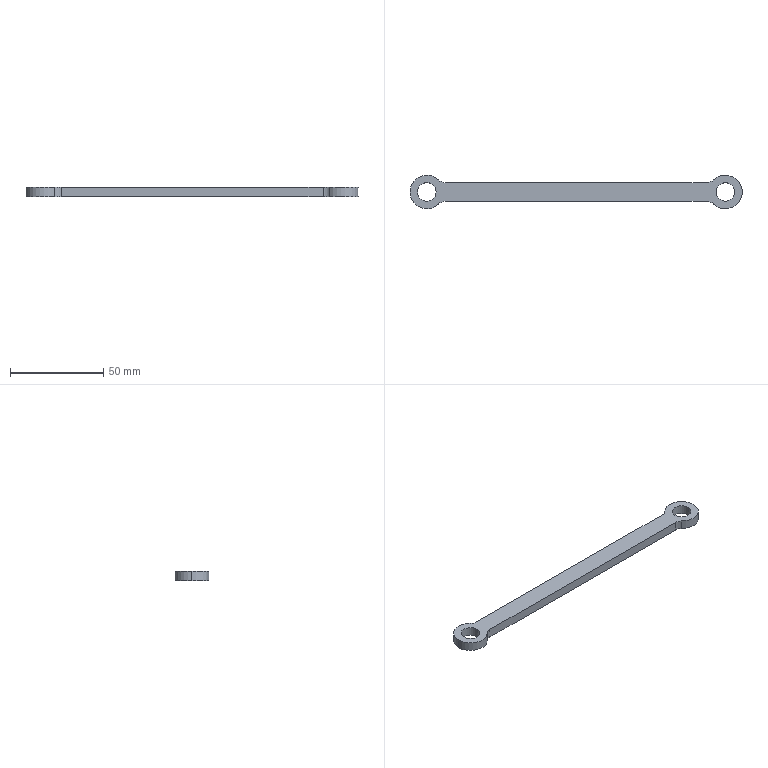Part | SolidWorks | features Extrusion 1 | 1 solid | 15 faces | box 178 x 18 x 5 mm | volume 8921 mm3 | cylinder 11 | plane 4 | commonest cylinder face diameters 10 x8 18 x3
STEP:
#1=CARTESIAN_POINT('',(155.,0.,5.));
#2=VERTEX_POINT('',#1);
#3=CARTESIAN_POINT('',(165.,0.,5.));
#4=VERTEX_POINT('',#3);
#5=CARTESIAN_POINT('',(160.,0.,5.));
#6=DIRECTION('',(0.,0.,1.));
#7=DIRECTION('',(1.,0.,0.));
#8=AXIS2_PLACEMENT_3D('',#5,#6,#7);
#9=CIRCLE('',#8,5.);
#10=EDGE_CURVE('',#2,#4,#9,.T.);
#11=ORIENTED_EDGE('',*,*,#10,.T.);
#12=CARTESIAN_POINT('',(165.,0.,0.));
#13=VERTEX_POINT('',#12);
#14=CARTESIAN_POINT('',(165.,0.,5.));
#15=DIRECTION('',(0.,0.,-1.));
#16=VECTOR('',#15,1000.);
#17=LINE('',#14,#16);
#18=EDGE_CURVE('',#4,#13,#17,.T.);
#19=ORIENTED_EDGE('',*,*,#18,.T.);
#20=CARTESIAN_POINT('',(155.,0.,0.));
#21=VERTEX_POINT('',#20);
#22=CARTESIAN_POINT('',(160.,0.,0.));
#23=DIRECTION('',(0.,0.,1.));
#24=DIRECTION('',(1.,0.,0.));
#25=AXIS2_PLACEMENT_3D('',#22,#23,#24);
#26=CIRCLE('',#25,5.);
#27=EDGE_CURVE('',#21,#13,#26,.T.);
#28=ORIENTED_EDGE('',*,*,#27,.F.);
#29=CARTESIAN_POINT('',(155.,0.,5.));
#30=DIRECTION('',(0.,0.,-1.));
#31=VECTOR('',#30,1000.);
#32=LINE('',#29,#31);
#33=EDGE_CURVE('',#2,#21,#32,.T.);
#34=ORIENTED_EDGE('',*,*,#33,.F.);
#35=EDGE_LOOP('',(#11,#19,#28,#34));
#36=FACE_OUTER_BOUND('',#35,.T.);
#37=CARTESIAN_POINT('',(160.,0.,5.));
#38=DIRECTION('',(0.,0.,-1.));
#39=DIRECTION('',(-1.,0.,0.));
#40=AXIS2_PLACEMENT_3D('',#37,#38,#39);
#41=CYLINDRICAL_SURFACE('',#40,5.);
#42=ADVANCED_FACE('',(#36),#41,.F.);
#43=CARTESIAN_POINT('',(-5.,0.,5.));
#44=VERTEX_POINT('',#43);
#45=CARTESIAN_POINT('',(5.,0.,5.));
#46=VERTEX_POINT('',#45);
#47=CARTESIAN_POINT('',(0.,0.,5.));
#48=DIRECTION('',(0.,0.,1.));
#49=DIRECTION('',(1.,0.,0.));
#50=AXIS2_PLACEMENT_3D('',#47,#48,#49);
#51=CIRCLE('',#50,5.);
#52=EDGE_CURVE('',#44,#46,#51,.T.);
#53=ORIENTED_EDGE('',*,*,#52,.T.);
#54=CARTESIAN_POINT('',(5.,0.,0.));
#55=VERTEX_POINT('',#54);
#56=CARTESIAN_POINT('',(5.,0.,5.));
#57=DIRECTION('',(0.,0.,-1.));
#58=VECTOR('',#57,1000.);
#59=LINE('',#56,#58);
#60=EDGE_CURVE('',#46,#55,#59,.T.);
#61=ORIENTED_EDGE('',*,*,#60,.T.);
#62=CARTESIAN_POINT('',(-5.,0.,0.));
#63=VERTEX_POINT('',#62);
#64=CARTESIAN_POINT('',(0.,0.,0.));
#65=DIRECTION('',(0.,0.,1.));
#66=DIRECTION('',(1.,0.,0.));
#67=AXIS2_PLACEMENT_3D('',#64,#65,#66);
#68=CIRCLE('',#67,5.);
#69=EDGE_CURVE('',#63,#55,#68,.T.);
#70=ORIENTED_EDGE('',*,*,#69,.F.);
#71=CARTESIAN_POINT('',(-5.,0.,5.));
#72=DIRECTION('',(0.,0.,-1.));
#73=VECTOR('',#72,1000.);
#74=LINE('',#71,#73);
#75=EDGE_CURVE('',#44,#63,#74,.T.);
#76=ORIENTED_EDGE('',*,*,#75,.F.);
#77=EDGE_LOOP('',(#53,#61,#70,#76));
#78=FACE_OUTER_BOUND('',#77,.T.);
#79=CARTESIAN_POINT('',(0.,0.,5.));
#80=DIRECTION('',(0.,0.,-1.));
#81=DIRECTION('',(-1.,0.,0.));
#82=AXIS2_PLACEMENT_3D('',#79,#80,#81);
#83=CYLINDRICAL_SURFACE('',#82,5.);
#84=ADVANCED_FACE('',(#78),#83,.F.);
#85=CARTESIAN_POINT('',(-9.,0.,5.));
#86=VERTEX_POINT('',#85);
#87=CARTESIAN_POINT('',(6.299,-6.429,5.));
#88=VERTEX_POINT('',#87);
#89=CARTESIAN_POINT('',(0.,0.,5.));
#90=DIRECTION('',(0.,0.,1.));
#91=DIRECTION('',(1.,0.,0.));
#92=AXIS2_PLACEMENT_3D('',#89,#90,#91);
#93=CIRCLE('',#92,9.);
#94=EDGE_CURVE('',#86,#88,#93,.T.);
#95=ORIENTED_EDGE('',*,*,#94,.F.);
#96=CARTESIAN_POINT('',(-9.,0.,0.));
#97=VERTEX_POINT('',#96);
#98=CARTESIAN_POINT('',(-9.,0.,5.));
#99=DIRECTION('',(0.,0.,-1.));
#100=VECTOR('',#99,1000.);
#101=LINE('',#98,#100);
#102=EDGE_CURVE('',#86,#97,#101,.T.);
#103=ORIENTED_EDGE('',*,*,#102,.T.);
#104=CARTESIAN_POINT('',(6.299,-6.429,0.));
#105=VERTEX_POINT('',#104);
#106=CARTESIAN_POINT('',(0.,0.,0.));
#107=DIRECTION('',(0.,0.,1.));
#108=DIRECTION('',(1.,0.,0.));
#109=AXIS2_PLACEMENT_3D('',#106,#107,#108);
#110=CIRCLE('',#109,9.);
#111=EDGE_CURVE('',#97,#105,#110,.T.);
#112=ORIENTED_EDGE('',*,*,#111,.T.);
#113=CARTESIAN_POINT('',(6.299,-6.429,5.));
#114=DIRECTION('',(0.,0.,-1.));
#115=VECTOR('',#114,1000.);
#116=LINE('',#113,#115);
#117=EDGE_CURVE('',#88,#105,#116,.T.);
#118=ORIENTED_EDGE('',*,*,#117,.F.);
#119=EDGE_LOOP('',(#95,#103,#112,#118));
#120=FACE_OUTER_BOUND('',#119,.T.);
#121=CARTESIAN_POINT('',(0.,0.,5.));
#122=DIRECTION('',(0.,0.,-1.));
#123=DIRECTION('',(-1.,0.,0.));
#124=AXIS2_PLACEMENT_3D('',#121,#122,#123);
#125=CYLINDRICAL_SURFACE('',#124,9.);
#126=ADVANCED_FACE('',(#120),#125,.T.);
#127=ORIENTED_EDGE('',*,*,#52,.F.);
#128=CARTESIAN_POINT('',(0.,0.,5.));
#129=DIRECTION('',(0.,0.,1.));
#130=DIRECTION('',(1.,0.,0.));
#131=AXIS2_PLACEMENT_3D('',#128,#129,#130);
#132=CIRCLE('',#131,5.);
#133=EDGE_CURVE('',#46,#44,#132,.T.);
#134=ORIENTED_EDGE('',*,*,#133,.F.);
#135=EDGE_LOOP('',(#127,#134));
#136=FACE_BOUND('',#135,.T.);
#137=CARTESIAN_POINT('',(153.701,6.429,5.));
#138=VERTEX_POINT('',#137);
#139=CARTESIAN_POINT('',(150.202,5.,5.));
#140=VERTEX_POINT('',#139);
#141=CARTESIAN_POINT('',(150.202,10.,5.));
#142=DIRECTION('',(0.,0.,-1.));
#143=DIRECTION('',(1.,0.,0.));
#144=AXIS2_PLACEMENT_3D('',#141,#142,#143);
#145=CIRCLE('',#144,5.);
#146=EDGE_CURVE('',#138,#140,#145,.T.);
#147=ORIENTED_EDGE('',*,*,#146,.T.);
#148=CARTESIAN_POINT('',(9.798,5.,5.));
#149=VERTEX_POINT('',#148);
#150=CARTESIAN_POINT('',(9.798,5.,5.));
#151=DIRECTION('',(-1.,0.,0.));
#152=VECTOR('',#151,1000.);
#153=LINE('',#150,#152);
#154=EDGE_CURVE('',#140,#149,#153,.T.);
#155=ORIENTED_EDGE('',*,*,#154,.T.);
#156=CARTESIAN_POINT('',(6.299,6.429,5.));
#157=VERTEX_POINT('',#156);
#158=CARTESIAN_POINT('',(9.798,10.,5.));
#159=DIRECTION('',(0.,0.,-1.));
#160=DIRECTION('',(-1.,0.,0.));
#161=AXIS2_PLACEMENT_3D('',#158,#159,#160);
#162=CIRCLE('',#161,5.);
#163=EDGE_CURVE('',#149,#157,#162,.T.);
#164=ORIENTED_EDGE('',*,*,#163,.T.);
#165=CARTESIAN_POINT('',(0.,0.,5.));
#166=DIRECTION('',(0.,0.,1.));
#167=DIRECTION('',(1.,0.,0.));
#168=AXIS2_PLACEMENT_3D('',#165,#166,#167);
#169=CIRCLE('',#168,9.);
#170=EDGE_CURVE('',#157,#86,#169,.T.);
#171=ORIENTED_EDGE('',*,*,#170,.T.);
#172=ORIENTED_EDGE('',*,*,#94,.T.);
#173=CARTESIAN_POINT('',(9.798,-5.,5.));
#174=VERTEX_POINT('',#173);
#175=CARTESIAN_POINT('',(9.798,-10.,5.));
#176=DIRECTION('',(0.,0.,-1.));
#177=DIRECTION('',(1.,0.,0.));
#178=AXIS2_PLACEMENT_3D('',#175,#176,#177);
#179=CIRCLE('',#178,5.);
#180=EDGE_CURVE('',#88,#174,#179,.T.);
#181=ORIENTED_EDGE('',*,*,#180,.T.);
#182=CARTESIAN_POINT('',(150.202,-5.,5.));
#183=VERTEX_POINT('',#182);
#184=CARTESIAN_POINT('',(9.798,-5.,5.));
#185=DIRECTION('',(1.,0.,0.));
#186=VECTOR('',#185,1000.);
#187=LINE('',#184,#186);
#188=EDGE_CURVE('',#174,#183,#187,.T.);
#189=ORIENTED_EDGE('',*,*,#188,.T.);
#190=CARTESIAN_POINT('',(153.701,-6.429,5.));
#191=VERTEX_POINT('',#190);
#192=CARTESIAN_POINT('',(150.202,-10.,5.));
#193=DIRECTION('',(0.,0.,-1.));
#194=DIRECTION('',(-1.,0.,0.));
#195=AXIS2_PLACEMENT_3D('',#192,#193,#194);
#196=CIRCLE('',#195,5.);
#197=EDGE_CURVE('',#183,#191,#196,.T.);
#198=ORIENTED_EDGE('',*,*,#197,.T.);
#199=CARTESIAN_POINT('',(160.,0.,5.));
#200=DIRECTION('',(0.,0.,1.));
#201=DIRECTION('',(1.,0.,0.));
#202=AXIS2_PLACEMENT_3D('',#199,#200,#201);
#203=CIRCLE('',#202,9.);
#204=EDGE_CURVE('',#191,#138,#203,.T.);
#205=ORIENTED_EDGE('',*,*,#204,.T.);
#206=EDGE_LOOP('',(#147,#155,#164,#171,#172,#181,#189,#198,#205));
#207=FACE_OUTER_BOUND('',#206,.T.);
#208=ORIENTED_EDGE('',*,*,#10,.F.);
#209=CARTESIAN_POINT('',(160.,0.,5.));
#210=DIRECTION('',(0.,0.,1.));
#211=DIRECTION('',(1.,0.,0.));
#212=AXIS2_PLACEMENT_3D('',#209,#210,#211);
#213=CIRCLE('',#212,5.);
#214=EDGE_CURVE('',#4,#2,#213,.T.);
#215=ORIENTED_EDGE('',*,*,#214,.F.);
#216=EDGE_LOOP('',(#208,#215));
#217=FACE_BOUND('',#216,.T.);
#218=CARTESIAN_POINT('',(150.202,10.,5.));
#219=DIRECTION('',(0.,0.,1.));
#220=DIRECTION('',(1.,0.,0.));
#221=AXIS2_PLACEMENT_3D('',#218,#219,#220);
#222=PLANE('',#221);
#223=ADVANCED_FACE('',(#136,#207,#217),#222,.T.);
#224=CARTESIAN_POINT('',(153.701,6.429,0.));
#225=VERTEX_POINT('',#224);
#226=CARTESIAN_POINT('',(150.202,5.,0.));
#227=VERTEX_POINT('',#226);
#228=CARTESIAN_POINT('',(150.202,10.,0.));
#229=DIRECTION('',(0.,0.,-1.));
#230=DIRECTION('',(1.,0.,0.));
#231=AXIS2_PLACEMENT_3D('',#228,#229,#230);
#232=CIRCLE('',#231,5.);
#233=EDGE_CURVE('',#225,#227,#232,.T.);
#234=ORIENTED_EDGE('',*,*,#233,.F.);
#235=CARTESIAN_POINT('',(153.701,-6.429,0.));
#236=VERTEX_POINT('',#235);
#237=CARTESIAN_POINT('',(160.,0.,0.));
#238=DIRECTION('',(0.,0.,1.));
#239=DIRECTION('',(1.,0.,0.));
#240=AXIS2_PLACEMENT_3D('',#237,#238,#239);
#241=CIRCLE('',#240,9.);
#242=EDGE_CURVE('',#236,#225,#241,.T.);
#243=ORIENTED_EDGE('',*,*,#242,.F.);
#244=CARTESIAN_POINT('',(150.202,-5.,0.));
#245=VERTEX_POINT('',#244);
#246=CARTESIAN_POINT('',(150.202,-10.,0.));
#247=DIRECTION('',(0.,0.,-1.));
#248=DIRECTION('',(-1.,0.,0.));
#249=AXIS2_PLACEMENT_3D('',#246,#247,#248);
#250=CIRCLE('',#249,5.);
#251=EDGE_CURVE('',#245,#236,#250,.T.);
#252=ORIENTED_EDGE('',*,*,#251,.F.);
#253=CARTESIAN_POINT('',(9.798,-5.,0.));
#254=VERTEX_POINT('',#253);
#255=CARTESIAN_POINT('',(9.798,-5.,0.));
#256=DIRECTION('',(1.,0.,0.));
#257=VECTOR('',#256,1000.);
#258=LINE('',#255,#257);
#259=EDGE_CURVE('',#254,#245,#258,.T.);
#260=ORIENTED_EDGE('',*,*,#259,.F.);
#261=CARTESIAN_POINT('',(9.798,-10.,0.));
#262=DIRECTION('',(0.,0.,-1.));
#263=DIRECTION('',(1.,0.,0.));
#264=AXIS2_PLACEMENT_3D('',#261,#262,#263);
#265=CIRCLE('',#264,5.);
#266=EDGE_CURVE('',#105,#254,#265,.T.);
#267=ORIENTED_EDGE('',*,*,#266,.F.);
#268=ORIENTED_EDGE('',*,*,#111,.F.);
#269=CARTESIAN_POINT('',(6.299,6.429,0.));
#270=VERTEX_POINT('',#269);
#271=CARTESIAN_POINT('',(0.,0.,0.));
#272=DIRECTION('',(0.,0.,1.));
#273=DIRECTION('',(1.,0.,0.));
#274=AXIS2_PLACEMENT_3D('',#271,#272,#273);
#275=CIRCLE('',#274,9.);
#276=EDGE_CURVE('',#270,#97,#275,.T.);
#277=ORIENTED_EDGE('',*,*,#276,.F.);
#278=CARTESIAN_POINT('',(9.798,5.,0.));
#279=VERTEX_POINT('',#278);
#280=CARTESIAN_POINT('',(9.798,10.,0.));
#281=DIRECTION('',(0.,0.,-1.));
#282=DIRECTION('',(-1.,0.,0.));
#283=AXIS2_PLACEMENT_3D('',#280,#281,#282);
#284=CIRCLE('',#283,5.);
#285=EDGE_CURVE('',#279,#270,#284,.T.);
#286=ORIENTED_EDGE('',*,*,#285,.F.);
#287=CARTESIAN_POINT('',(9.798,5.,0.));
#288=DIRECTION('',(-1.,0.,0.));
#289=VECTOR('',#288,1000.);
#290=LINE('',#287,#289);
#291=EDGE_CURVE('',#227,#279,#290,.T.);
#292=ORIENTED_EDGE('',*,*,#291,.F.);
#293=EDGE_LOOP('',(#234,#243,#252,#260,#267,#268,#277,#286,#292));
#294=FACE_OUTER_BOUND('',#293,.T.);
#295=ORIENTED_EDGE('',*,*,#69,.T.);
#296=CARTESIAN_POINT('',(0.,0.,0.));
#297=DIRECTION('',(0.,0.,1.));
#298=DIRECTION('',(1.,0.,0.));
#299=AXIS2_PLACEMENT_3D('',#296,#297,#298);
#300=CIRCLE('',#299,5.);
#301=EDGE_CURVE('',#55,#63,#300,.T.);
#302=ORIENTED_EDGE('',*,*,#301,.T.);
#303=EDGE_LOOP('',(#295,#302));
#304=FACE_BOUND('',#303,.T.);
#305=ORIENTED_EDGE('',*,*,#27,.T.);
#306=CARTESIAN_POINT('',(160.,0.,0.));
#307=DIRECTION('',(0.,0.,1.));
#308=DIRECTION('',(1.,0.,0.));
#309=AXIS2_PLACEMENT_3D('',#306,#307,#308);
#310=CIRCLE('',#309,5.);
#311=EDGE_CURVE('',#13,#21,#310,.T.);
#312=ORIENTED_EDGE('',*,*,#311,.T.);
#313=EDGE_LOOP('',(#305,#312));
#314=FACE_BOUND('',#313,.T.);
#315=CARTESIAN_POINT('',(150.202,10.,0.));
#316=DIRECTION('',(0.,0.,1.));
#317=DIRECTION('',(1.,0.,0.));
#318=AXIS2_PLACEMENT_3D('',#315,#316,#317);
#319=PLANE('',#318);
#320=ADVANCED_FACE('',(#294,#304,#314),#319,.F.);
#321=ORIENTED_EDGE('',*,*,#233,.T.);
#322=CARTESIAN_POINT('',(150.202,5.,5.));
#323=DIRECTION('',(0.,0.,-1.));
#324=VECTOR('',#323,1000.);
#325=LINE('',#322,#324);
#326=EDGE_CURVE('',#140,#227,#325,.T.);
#327=ORIENTED_EDGE('',*,*,#326,.F.);
#328=ORIENTED_EDGE('',*,*,#146,.F.);
#329=CARTESIAN_POINT('',(153.701,6.429,5.));
#330=DIRECTION('',(0.,0.,-1.));
#331=VECTOR('',#330,1000.);
#332=LINE('',#329,#331);
#333=EDGE_CURVE('',#138,#225,#332,.T.);
#334=ORIENTED_EDGE('',*,*,#333,.T.);
#335=EDGE_LOOP('',(#321,#327,#328,#334));
#336=FACE_OUTER_BOUND('',#335,.T.);
#337=CARTESIAN_POINT('',(150.202,10.,5.));
#338=DIRECTION('',(0.,0.,-1.));
#339=DIRECTION('',(-1.,0.,0.));
#340=AXIS2_PLACEMENT_3D('',#337,#338,#339);
#341=CYLINDRICAL_SURFACE('',#340,5.);
#342=ADVANCED_FACE('',(#336),#341,.F.);
#343=ORIENTED_EDGE('',*,*,#291,.T.);
#344=CARTESIAN_POINT('',(9.798,5.,5.));
#345=DIRECTION('',(0.,0.,-1.));
#346=VECTOR('',#345,1000.);
#347=LINE('',#344,#346);
#348=EDGE_CURVE('',#149,#279,#347,.T.);
#349=ORIENTED_EDGE('',*,*,#348,.F.);
#350=ORIENTED_EDGE('',*,*,#154,.F.);
#351=ORIENTED_EDGE('',*,*,#326,.T.);
#352=EDGE_LOOP('',(#343,#349,#350,#351));
#353=FACE_OUTER_BOUND('',#352,.T.);
#354=CARTESIAN_POINT('',(9.798,5.,5.));
#355=DIRECTION('',(0.,-1.,0.));
#356=DIRECTION('',(0.,0.,-1.));
#357=AXIS2_PLACEMENT_3D('',#354,#355,#356);
#358=PLANE('',#357);
#359=ADVANCED_FACE('',(#353),#358,.F.);
#360=ORIENTED_EDGE('',*,*,#285,.T.);
#361=CARTESIAN_POINT('',(6.299,6.429,5.));
#362=DIRECTION('',(0.,0.,-1.));
#363=VECTOR('',#362,1000.);
#364=LINE('',#361,#363);
#365=EDGE_CURVE('',#157,#270,#364,.T.);
#366=ORIENTED_EDGE('',*,*,#365,.F.);
#367=ORIENTED_EDGE('',*,*,#163,.F.);
#368=ORIENTED_EDGE('',*,*,#348,.T.);
#369=EDGE_LOOP('',(#360,#366,#367,#368));
#370=FACE_OUTER_BOUND('',#369,.T.);
#371=CARTESIAN_POINT('',(9.798,10.,5.));
#372=DIRECTION('',(0.,0.,-1.));
#373=DIRECTION('',(-1.,0.,0.));
#374=AXIS2_PLACEMENT_3D('',#371,#372,#373);
#375=CYLINDRICAL_SURFACE('',#374,5.);
#376=ADVANCED_FACE('',(#370),#375,.F.);
#377=ORIENTED_EDGE('',*,*,#102,.F.);
#378=ORIENTED_EDGE('',*,*,#170,.F.);
#379=ORIENTED_EDGE('',*,*,#365,.T.);
#380=ORIENTED_EDGE('',*,*,#276,.T.);
#381=EDGE_LOOP('',(#377,#378,#379,#380));
#382=FACE_OUTER_BOUND('',#381,.T.);
#383=CARTESIAN_POINT('',(0.,0.,5.));
#384=DIRECTION('',(0.,0.,-1.));
#385=DIRECTION('',(-1.,0.,0.));
#386=AXIS2_PLACEMENT_3D('',#383,#384,#385);
#387=CYLINDRICAL_SURFACE('',#386,9.);
#388=ADVANCED_FACE('',(#382),#387,.T.);
#389=ORIENTED_EDGE('',*,*,#266,.T.);
#390=CARTESIAN_POINT('',(9.798,-5.,5.));
#391=DIRECTION('',(0.,0.,-1.));
#392=VECTOR('',#391,1000.);
#393=LINE('',#390,#392);
#394=EDGE_CURVE('',#174,#254,#393,.T.);
#395=ORIENTED_EDGE('',*,*,#394,.F.);
#396=ORIENTED_EDGE('',*,*,#180,.F.);
#397=ORIENTED_EDGE('',*,*,#117,.T.);
#398=EDGE_LOOP('',(#389,#395,#396,#397));
#399=FACE_OUTER_BOUND('',#398,.T.);
#400=CARTESIAN_POINT('',(9.798,-10.,5.));
#401=DIRECTION('',(0.,0.,-1.));
#402=DIRECTION('',(-1.,0.,0.));
#403=AXIS2_PLACEMENT_3D('',#400,#401,#402);
#404=CYLINDRICAL_SURFACE('',#403,5.);
#405=ADVANCED_FACE('',(#399),#404,.F.);
#406=ORIENTED_EDGE('',*,*,#259,.T.);
#407=CARTESIAN_POINT('',(150.202,-5.,5.));
#408=DIRECTION('',(0.,0.,-1.));
#409=VECTOR('',#408,1000.);
#410=LINE('',#407,#409);
#411=EDGE_CURVE('',#183,#245,#410,.T.);
#412=ORIENTED_EDGE('',*,*,#411,.F.);
#413=ORIENTED_EDGE('',*,*,#188,.F.);
#414=ORIENTED_EDGE('',*,*,#394,.T.);
#415=EDGE_LOOP('',(#406,#412,#413,#414));
#416=FACE_OUTER_BOUND('',#415,.T.);
#417=CARTESIAN_POINT('',(9.798,-5.,5.));
#418=DIRECTION('',(0.,1.,0.));
#419=DIRECTION('',(0.,0.,1.));
#420=AXIS2_PLACEMENT_3D('',#417,#418,#419);
#421=PLANE('',#420);
#422=ADVANCED_FACE('',(#416),#421,.F.);
#423=ORIENTED_EDGE('',*,*,#251,.T.);
#424=CARTESIAN_POINT('',(153.701,-6.429,5.));
#425=DIRECTION('',(0.,0.,-1.));
#426=VECTOR('',#425,1000.);
#427=LINE('',#424,#426);
#428=EDGE_CURVE('',#191,#236,#427,.T.);
#429=ORIENTED_EDGE('',*,*,#428,.F.);
#430=ORIENTED_EDGE('',*,*,#197,.F.);
#431=ORIENTED_EDGE('',*,*,#411,.T.);
#432=EDGE_LOOP('',(#423,#429,#430,#431));
#433=FACE_OUTER_BOUND('',#432,.T.);
#434=CARTESIAN_POINT('',(150.202,-10.,5.));
#435=DIRECTION('',(0.,0.,-1.));
#436=DIRECTION('',(-1.,0.,0.));
#437=AXIS2_PLACEMENT_3D('',#434,#435,#436);
#438=CYLINDRICAL_SURFACE('',#437,5.);
#439=ADVANCED_FACE('',(#433),#438,.F.);
#440=ORIENTED_EDGE('',*,*,#242,.T.);
#441=ORIENTED_EDGE('',*,*,#333,.F.);
#442=ORIENTED_EDGE('',*,*,#204,.F.);
#443=ORIENTED_EDGE('',*,*,#428,.T.);
#444=EDGE_LOOP('',(#440,#441,#442,#443));
#445=FACE_OUTER_BOUND('',#444,.T.);
#446=CARTESIAN_POINT('',(160.,0.,5.));
#447=DIRECTION('',(0.,0.,-1.));
#448=DIRECTION('',(-1.,0.,0.));
#449=AXIS2_PLACEMENT_3D('',#446,#447,#448);
#450=CYLINDRICAL_SURFACE('',#449,9.);
#451=ADVANCED_FACE('',(#445),#450,.T.);
#452=ORIENTED_EDGE('',*,*,#60,.F.);
#453=ORIENTED_EDGE('',*,*,#133,.T.);
#454=ORIENTED_EDGE('',*,*,#75,.T.);
#455=ORIENTED_EDGE('',*,*,#301,.F.);
#456=EDGE_LOOP('',(#452,#453,#454,#455));
#457=FACE_OUTER_BOUND('',#456,.T.);
#458=CARTESIAN_POINT('',(0.,0.,5.));
#459=DIRECTION('',(0.,0.,-1.));
#460=DIRECTION('',(-1.,0.,0.));
#461=AXIS2_PLACEMENT_3D('',#458,#459,#460);
#462=CYLINDRICAL_SURFACE('',#461,5.);
#463=ADVANCED_FACE('',(#457),#462,.F.);
#464=ORIENTED_EDGE('',*,*,#18,.F.);
#465=ORIENTED_EDGE('',*,*,#214,.T.);
#466=ORIENTED_EDGE('',*,*,#33,.T.);
#467=ORIENTED_EDGE('',*,*,#311,.F.);
#468=EDGE_LOOP('',(#464,#465,#466,#467));
#469=FACE_OUTER_BOUND('',#468,.T.);
#470=CARTESIAN_POINT('',(160.,0.,5.));
#471=DIRECTION('',(0.,0.,-1.));
#472=DIRECTION('',(-1.,0.,0.));
#473=AXIS2_PLACEMENT_3D('',#470,#471,#472);
#474=CYLINDRICAL_SURFACE('',#473,5.);
#475=ADVANCED_FACE('',(#469),#474,.F.);
#476=CLOSED_SHELL('',(#42,#84,#126,#223,#320,#342,#359,#376,#388,#405,#422,#439,#451,#463,#475));
#477=MANIFOLD_SOLID_BREP('',#476);
#478=CARTESIAN_POINT('',(0.,0.,0.));
#479=DIRECTION('',(0.,0.,1.));
#480=DIRECTION('',(1.,0.,0.));
#481=AXIS2_PLACEMENT_3D('',#478,#479,#480);
#482=(LENGTH_UNIT()NAMED_UNIT(*)SI_UNIT(.MILLI.,.METRE.));
#483=UNCERTAINTY_MEASURE_WITH_UNIT(LENGTH_MEASURE(0.00001),#482,'','');
#484=(NAMED_UNIT(*)PLANE_ANGLE_UNIT()SI_UNIT($,.RADIAN.));
#485=(NAMED_UNIT(*)SI_UNIT($,.STERADIAN.)SOLID_ANGLE_UNIT());
#486=(GEOMETRIC_REPRESENTATION_CONTEXT(3)GLOBAL_UNCERTAINTY_ASSIGNED_CONTEXT((#483))GLOBAL_UNIT_ASSIGNED_CONTEXT((#482,#484,#485))REPRESENTATION_CONTEXT('',''));
#487=ADVANCED_BREP_SHAPE_REPRESENTATION('',(#477,#481),#486);